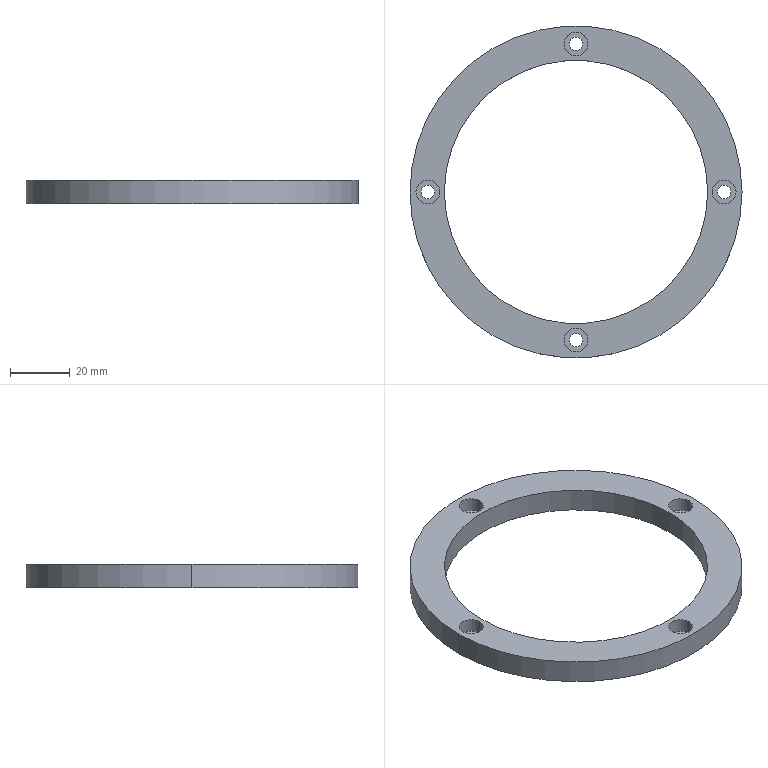Part | SolidWorks | features CirPattern 1, Extrusion 1, HoleWzd 1 | 1 solid | 26 faces | box 111 x 111 x 8 mm | volume 27617 mm3 | cylinder 20 | plane 6 | commonest cylinder face diameters 4.5 x8 8 x8 88 x2 111 x2
STEP:
#1=CARTESIAN_POINT('',(-53.5,0.,3.4));
#2=VERTEX_POINT('',#1);
#3=CARTESIAN_POINT('',(-45.5,0.,3.4));
#4=VERTEX_POINT('',#3);
#5=CARTESIAN_POINT('',(-49.5,0.,3.4));
#6=DIRECTION('',(0.,0.,1.));
#7=DIRECTION('',(1.,0.,0.));
#8=AXIS2_PLACEMENT_3D('',#5,#6,#7);
#9=CIRCLE('',#8,4.);
#10=EDGE_CURVE('',#2,#4,#9,.T.);
#11=ORIENTED_EDGE('',*,*,#10,.F.);
#12=CARTESIAN_POINT('',(-53.5,0.,8.));
#13=VERTEX_POINT('',#12);
#14=CARTESIAN_POINT('',(-53.5,0.,8.));
#15=DIRECTION('',(0.,0.,1.));
#16=VECTOR('',#15,1000.);
#17=LINE('',#14,#16);
#18=EDGE_CURVE('',#2,#13,#17,.T.);
#19=ORIENTED_EDGE('',*,*,#18,.T.);
#20=CARTESIAN_POINT('',(-45.5,0.,8.));
#21=VERTEX_POINT('',#20);
#22=CARTESIAN_POINT('',(-49.5,0.,8.));
#23=DIRECTION('',(0.,0.,1.));
#24=DIRECTION('',(1.,0.,0.));
#25=AXIS2_PLACEMENT_3D('',#22,#23,#24);
#26=CIRCLE('',#25,4.);
#27=EDGE_CURVE('',#13,#21,#26,.T.);
#28=ORIENTED_EDGE('',*,*,#27,.T.);
#29=CARTESIAN_POINT('',(-45.5,0.,8.));
#30=DIRECTION('',(0.,0.,1.));
#31=VECTOR('',#30,1000.);
#32=LINE('',#29,#31);
#33=EDGE_CURVE('',#4,#21,#32,.T.);
#34=ORIENTED_EDGE('',*,*,#33,.F.);
#35=EDGE_LOOP('',(#11,#19,#28,#34));
#36=FACE_OUTER_BOUND('',#35,.T.);
#37=CARTESIAN_POINT('',(-49.5,0.,8.));
#38=DIRECTION('',(0.,0.,1.));
#39=DIRECTION('',(1.,0.,0.));
#40=AXIS2_PLACEMENT_3D('',#37,#38,#39);
#41=CYLINDRICAL_SURFACE('',#40,4.);
#42=ADVANCED_FACE('',(#36),#41,.F.);
#43=CARTESIAN_POINT('',(-51.75,0.,0.));
#44=VERTEX_POINT('',#43);
#45=CARTESIAN_POINT('',(-47.25,0.,0.));
#46=VERTEX_POINT('',#45);
#47=CARTESIAN_POINT('',(-49.5,0.,0.));
#48=DIRECTION('',(0.,0.,1.));
#49=DIRECTION('',(1.,0.,0.));
#50=AXIS2_PLACEMENT_3D('',#47,#48,#49);
#51=CIRCLE('',#50,2.25);
#52=EDGE_CURVE('',#44,#46,#51,.T.);
#53=ORIENTED_EDGE('',*,*,#52,.F.);
#54=CARTESIAN_POINT('',(-51.75,0.,3.4));
#55=VERTEX_POINT('',#54);
#56=CARTESIAN_POINT('',(-51.75,0.,8.));
#57=DIRECTION('',(0.,0.,1.));
#58=VECTOR('',#57,1000.);
#59=LINE('',#56,#58);
#60=EDGE_CURVE('',#44,#55,#59,.T.);
#61=ORIENTED_EDGE('',*,*,#60,.T.);
#62=CARTESIAN_POINT('',(-47.25,0.,3.4));
#63=VERTEX_POINT('',#62);
#64=CARTESIAN_POINT('',(-49.5,0.,3.4));
#65=DIRECTION('',(0.,0.,1.));
#66=DIRECTION('',(1.,0.,0.));
#67=AXIS2_PLACEMENT_3D('',#64,#65,#66);
#68=CIRCLE('',#67,2.25);
#69=EDGE_CURVE('',#55,#63,#68,.T.);
#70=ORIENTED_EDGE('',*,*,#69,.T.);
#71=CARTESIAN_POINT('',(-47.25,0.,8.));
#72=DIRECTION('',(0.,0.,1.));
#73=VECTOR('',#72,1000.);
#74=LINE('',#71,#73);
#75=EDGE_CURVE('',#46,#63,#74,.T.);
#76=ORIENTED_EDGE('',*,*,#75,.F.);
#77=EDGE_LOOP('',(#53,#61,#70,#76));
#78=FACE_OUTER_BOUND('',#77,.T.);
#79=CARTESIAN_POINT('',(-49.5,0.,8.));
#80=DIRECTION('',(0.,0.,1.));
#81=DIRECTION('',(1.,0.,0.));
#82=AXIS2_PLACEMENT_3D('',#79,#80,#81);
#83=CYLINDRICAL_SURFACE('',#82,2.25);
#84=ADVANCED_FACE('',(#78),#83,.F.);
#85=CARTESIAN_POINT('',(-4.,-49.5,3.4));
#86=VERTEX_POINT('',#85);
#87=CARTESIAN_POINT('',(4.,-49.5,3.4));
#88=VERTEX_POINT('',#87);
#89=CARTESIAN_POINT('',(0.,-49.5,3.4));
#90=DIRECTION('',(0.,0.,1.));
#91=DIRECTION('',(1.,0.,0.));
#92=AXIS2_PLACEMENT_3D('',#89,#90,#91);
#93=CIRCLE('',#92,4.);
#94=EDGE_CURVE('',#86,#88,#93,.T.);
#95=ORIENTED_EDGE('',*,*,#94,.F.);
#96=CARTESIAN_POINT('',(-4.,-49.5,8.));
#97=VERTEX_POINT('',#96);
#98=CARTESIAN_POINT('',(-4.,-49.5,8.));
#99=DIRECTION('',(0.,0.,1.));
#100=VECTOR('',#99,1000.);
#101=LINE('',#98,#100);
#102=EDGE_CURVE('',#86,#97,#101,.T.);
#103=ORIENTED_EDGE('',*,*,#102,.T.);
#104=CARTESIAN_POINT('',(4.,-49.5,8.));
#105=VERTEX_POINT('',#104);
#106=CARTESIAN_POINT('',(0.,-49.5,8.));
#107=DIRECTION('',(0.,0.,1.));
#108=DIRECTION('',(1.,0.,0.));
#109=AXIS2_PLACEMENT_3D('',#106,#107,#108);
#110=CIRCLE('',#109,4.);
#111=EDGE_CURVE('',#97,#105,#110,.T.);
#112=ORIENTED_EDGE('',*,*,#111,.T.);
#113=CARTESIAN_POINT('',(4.,-49.5,8.));
#114=DIRECTION('',(0.,0.,1.));
#115=VECTOR('',#114,1000.);
#116=LINE('',#113,#115);
#117=EDGE_CURVE('',#88,#105,#116,.T.);
#118=ORIENTED_EDGE('',*,*,#117,.F.);
#119=EDGE_LOOP('',(#95,#103,#112,#118));
#120=FACE_OUTER_BOUND('',#119,.T.);
#121=CARTESIAN_POINT('',(0.,-49.5,8.));
#122=DIRECTION('',(0.,0.,1.));
#123=DIRECTION('',(1.,0.,0.));
#124=AXIS2_PLACEMENT_3D('',#121,#122,#123);
#125=CYLINDRICAL_SURFACE('',#124,4.);
#126=ADVANCED_FACE('',(#120),#125,.F.);
#127=CARTESIAN_POINT('',(-2.25,-49.5,0.));
#128=VERTEX_POINT('',#127);
#129=CARTESIAN_POINT('',(2.25,-49.5,0.));
#130=VERTEX_POINT('',#129);
#131=CARTESIAN_POINT('',(0.,-49.5,0.));
#132=DIRECTION('',(0.,0.,1.));
#133=DIRECTION('',(1.,0.,0.));
#134=AXIS2_PLACEMENT_3D('',#131,#132,#133);
#135=CIRCLE('',#134,2.25);
#136=EDGE_CURVE('',#128,#130,#135,.T.);
#137=ORIENTED_EDGE('',*,*,#136,.F.);
#138=CARTESIAN_POINT('',(-2.25,-49.5,3.4));
#139=VERTEX_POINT('',#138);
#140=CARTESIAN_POINT('',(-2.25,-49.5,8.));
#141=DIRECTION('',(0.,0.,1.));
#142=VECTOR('',#141,1000.);
#143=LINE('',#140,#142);
#144=EDGE_CURVE('',#128,#139,#143,.T.);
#145=ORIENTED_EDGE('',*,*,#144,.T.);
#146=CARTESIAN_POINT('',(2.25,-49.5,3.4));
#147=VERTEX_POINT('',#146);
#148=CARTESIAN_POINT('',(0.,-49.5,3.4));
#149=DIRECTION('',(0.,0.,1.));
#150=DIRECTION('',(1.,0.,0.));
#151=AXIS2_PLACEMENT_3D('',#148,#149,#150);
#152=CIRCLE('',#151,2.25);
#153=EDGE_CURVE('',#139,#147,#152,.T.);
#154=ORIENTED_EDGE('',*,*,#153,.T.);
#155=CARTESIAN_POINT('',(2.25,-49.5,8.));
#156=DIRECTION('',(0.,0.,1.));
#157=VECTOR('',#156,1000.);
#158=LINE('',#155,#157);
#159=EDGE_CURVE('',#130,#147,#158,.T.);
#160=ORIENTED_EDGE('',*,*,#159,.F.);
#161=EDGE_LOOP('',(#137,#145,#154,#160));
#162=FACE_OUTER_BOUND('',#161,.T.);
#163=CARTESIAN_POINT('',(0.,-49.5,8.));
#164=DIRECTION('',(0.,0.,1.));
#165=DIRECTION('',(1.,0.,0.));
#166=AXIS2_PLACEMENT_3D('',#163,#164,#165);
#167=CYLINDRICAL_SURFACE('',#166,2.25);
#168=ADVANCED_FACE('',(#162),#167,.F.);
#169=CARTESIAN_POINT('',(45.5,0.,3.4));
#170=VERTEX_POINT('',#169);
#171=CARTESIAN_POINT('',(53.5,0.,3.4));
#172=VERTEX_POINT('',#171);
#173=CARTESIAN_POINT('',(49.5,0.,3.4));
#174=DIRECTION('',(0.,0.,1.));
#175=DIRECTION('',(1.,0.,0.));
#176=AXIS2_PLACEMENT_3D('',#173,#174,#175);
#177=CIRCLE('',#176,4.);
#178=EDGE_CURVE('',#170,#172,#177,.T.);
#179=ORIENTED_EDGE('',*,*,#178,.F.);
#180=CARTESIAN_POINT('',(45.5,0.,8.));
#181=VERTEX_POINT('',#180);
#182=CARTESIAN_POINT('',(45.5,0.,8.));
#183=DIRECTION('',(0.,0.,1.));
#184=VECTOR('',#183,1000.);
#185=LINE('',#182,#184);
#186=EDGE_CURVE('',#170,#181,#185,.T.);
#187=ORIENTED_EDGE('',*,*,#186,.T.);
#188=CARTESIAN_POINT('',(53.5,0.,8.));
#189=VERTEX_POINT('',#188);
#190=CARTESIAN_POINT('',(49.5,0.,8.));
#191=DIRECTION('',(0.,0.,1.));
#192=DIRECTION('',(1.,0.,0.));
#193=AXIS2_PLACEMENT_3D('',#190,#191,#192);
#194=CIRCLE('',#193,4.);
#195=EDGE_CURVE('',#181,#189,#194,.T.);
#196=ORIENTED_EDGE('',*,*,#195,.T.);
#197=CARTESIAN_POINT('',(53.5,0.,8.));
#198=DIRECTION('',(0.,0.,1.));
#199=VECTOR('',#198,1000.);
#200=LINE('',#197,#199);
#201=EDGE_CURVE('',#172,#189,#200,.T.);
#202=ORIENTED_EDGE('',*,*,#201,.F.);
#203=EDGE_LOOP('',(#179,#187,#196,#202));
#204=FACE_OUTER_BOUND('',#203,.T.);
#205=CARTESIAN_POINT('',(49.5,0.,8.));
#206=DIRECTION('',(0.,0.,1.));
#207=DIRECTION('',(1.,0.,0.));
#208=AXIS2_PLACEMENT_3D('',#205,#206,#207);
#209=CYLINDRICAL_SURFACE('',#208,4.);
#210=ADVANCED_FACE('',(#204),#209,.F.);
#211=CARTESIAN_POINT('',(47.25,0.,0.));
#212=VERTEX_POINT('',#211);
#213=CARTESIAN_POINT('',(51.75,0.,0.));
#214=VERTEX_POINT('',#213);
#215=CARTESIAN_POINT('',(49.5,0.,0.));
#216=DIRECTION('',(0.,0.,1.));
#217=DIRECTION('',(1.,0.,0.));
#218=AXIS2_PLACEMENT_3D('',#215,#216,#217);
#219=CIRCLE('',#218,2.25);
#220=EDGE_CURVE('',#212,#214,#219,.T.);
#221=ORIENTED_EDGE('',*,*,#220,.F.);
#222=CARTESIAN_POINT('',(47.25,0.,3.4));
#223=VERTEX_POINT('',#222);
#224=CARTESIAN_POINT('',(47.25,0.,8.));
#225=DIRECTION('',(0.,0.,1.));
#226=VECTOR('',#225,1000.);
#227=LINE('',#224,#226);
#228=EDGE_CURVE('',#212,#223,#227,.T.);
#229=ORIENTED_EDGE('',*,*,#228,.T.);
#230=CARTESIAN_POINT('',(51.75,0.,3.4));
#231=VERTEX_POINT('',#230);
#232=CARTESIAN_POINT('',(49.5,0.,3.4));
#233=DIRECTION('',(0.,0.,1.));
#234=DIRECTION('',(1.,0.,0.));
#235=AXIS2_PLACEMENT_3D('',#232,#233,#234);
#236=CIRCLE('',#235,2.25);
#237=EDGE_CURVE('',#223,#231,#236,.T.);
#238=ORIENTED_EDGE('',*,*,#237,.T.);
#239=CARTESIAN_POINT('',(51.75,0.,8.));
#240=DIRECTION('',(0.,0.,1.));
#241=VECTOR('',#240,1000.);
#242=LINE('',#239,#241);
#243=EDGE_CURVE('',#214,#231,#242,.T.);
#244=ORIENTED_EDGE('',*,*,#243,.F.);
#245=EDGE_LOOP('',(#221,#229,#238,#244));
#246=FACE_OUTER_BOUND('',#245,.T.);
#247=CARTESIAN_POINT('',(49.5,0.,8.));
#248=DIRECTION('',(0.,0.,1.));
#249=DIRECTION('',(1.,0.,0.));
#250=AXIS2_PLACEMENT_3D('',#247,#248,#249);
#251=CYLINDRICAL_SURFACE('',#250,2.25);
#252=ADVANCED_FACE('',(#246),#251,.F.);
#253=CARTESIAN_POINT('',(-4.,49.5,3.4));
#254=VERTEX_POINT('',#253);
#255=CARTESIAN_POINT('',(4.,49.5,3.4));
#256=VERTEX_POINT('',#255);
#257=CARTESIAN_POINT('',(0.,49.5,3.4));
#258=DIRECTION('',(0.,0.,1.));
#259=DIRECTION('',(1.,0.,0.));
#260=AXIS2_PLACEMENT_3D('',#257,#258,#259);
#261=CIRCLE('',#260,4.);
#262=EDGE_CURVE('',#254,#256,#261,.T.);
#263=ORIENTED_EDGE('',*,*,#262,.F.);
#264=CARTESIAN_POINT('',(-4.,49.5,8.));
#265=VERTEX_POINT('',#264);
#266=CARTESIAN_POINT('',(-4.,49.5,8.));
#267=DIRECTION('',(0.,0.,1.));
#268=VECTOR('',#267,1000.);
#269=LINE('',#266,#268);
#270=EDGE_CURVE('',#254,#265,#269,.T.);
#271=ORIENTED_EDGE('',*,*,#270,.T.);
#272=CARTESIAN_POINT('',(4.,49.5,8.));
#273=VERTEX_POINT('',#272);
#274=CARTESIAN_POINT('',(0.,49.5,8.));
#275=DIRECTION('',(0.,0.,1.));
#276=DIRECTION('',(1.,0.,0.));
#277=AXIS2_PLACEMENT_3D('',#274,#275,#276);
#278=CIRCLE('',#277,4.);
#279=EDGE_CURVE('',#265,#273,#278,.T.);
#280=ORIENTED_EDGE('',*,*,#279,.T.);
#281=CARTESIAN_POINT('',(4.,49.5,8.));
#282=DIRECTION('',(0.,0.,1.));
#283=VECTOR('',#282,1000.);
#284=LINE('',#281,#283);
#285=EDGE_CURVE('',#256,#273,#284,.T.);
#286=ORIENTED_EDGE('',*,*,#285,.F.);
#287=EDGE_LOOP('',(#263,#271,#280,#286));
#288=FACE_OUTER_BOUND('',#287,.T.);
#289=CARTESIAN_POINT('',(0.,49.5,8.));
#290=DIRECTION('',(0.,0.,1.));
#291=DIRECTION('',(1.,0.,0.));
#292=AXIS2_PLACEMENT_3D('',#289,#290,#291);
#293=CYLINDRICAL_SURFACE('',#292,4.);
#294=ADVANCED_FACE('',(#288),#293,.F.);
#295=CARTESIAN_POINT('',(-2.25,49.5,0.));
#296=VERTEX_POINT('',#295);
#297=CARTESIAN_POINT('',(2.25,49.5,0.));
#298=VERTEX_POINT('',#297);
#299=CARTESIAN_POINT('',(0.,49.5,0.));
#300=DIRECTION('',(0.,0.,1.));
#301=DIRECTION('',(1.,0.,0.));
#302=AXIS2_PLACEMENT_3D('',#299,#300,#301);
#303=CIRCLE('',#302,2.25);
#304=EDGE_CURVE('',#296,#298,#303,.T.);
#305=ORIENTED_EDGE('',*,*,#304,.F.);
#306=CARTESIAN_POINT('',(-2.25,49.5,3.4));
#307=VERTEX_POINT('',#306);
#308=CARTESIAN_POINT('',(-2.25,49.5,8.));
#309=DIRECTION('',(0.,0.,1.));
#310=VECTOR('',#309,1000.);
#311=LINE('',#308,#310);
#312=EDGE_CURVE('',#296,#307,#311,.T.);
#313=ORIENTED_EDGE('',*,*,#312,.T.);
#314=CARTESIAN_POINT('',(2.25,49.5,3.4));
#315=VERTEX_POINT('',#314);
#316=CARTESIAN_POINT('',(0.,49.5,3.4));
#317=DIRECTION('',(0.,0.,1.));
#318=DIRECTION('',(1.,0.,0.));
#319=AXIS2_PLACEMENT_3D('',#316,#317,#318);
#320=CIRCLE('',#319,2.25);
#321=EDGE_CURVE('',#307,#315,#320,.T.);
#322=ORIENTED_EDGE('',*,*,#321,.T.);
#323=CARTESIAN_POINT('',(2.25,49.5,8.));
#324=DIRECTION('',(0.,0.,1.));
#325=VECTOR('',#324,1000.);
#326=LINE('',#323,#325);
#327=EDGE_CURVE('',#298,#315,#326,.T.);
#328=ORIENTED_EDGE('',*,*,#327,.F.);
#329=EDGE_LOOP('',(#305,#313,#322,#328));
#330=FACE_OUTER_BOUND('',#329,.T.);
#331=CARTESIAN_POINT('',(0.,49.5,8.));
#332=DIRECTION('',(0.,0.,1.));
#333=DIRECTION('',(1.,0.,0.));
#334=AXIS2_PLACEMENT_3D('',#331,#332,#333);
#335=CYLINDRICAL_SURFACE('',#334,2.25);
#336=ADVANCED_FACE('',(#330),#335,.F.);
#337=CARTESIAN_POINT('',(-44.,0.,8.));
#338=VERTEX_POINT('',#337);
#339=CARTESIAN_POINT('',(44.,0.,8.));
#340=VERTEX_POINT('',#339);
#341=CARTESIAN_POINT('',(0.,0.,8.));
#342=DIRECTION('',(0.,0.,1.));
#343=DIRECTION('',(1.,0.,0.));
#344=AXIS2_PLACEMENT_3D('',#341,#342,#343);
#345=CIRCLE('',#344,44.);
#346=EDGE_CURVE('',#338,#340,#345,.T.);
#347=ORIENTED_EDGE('',*,*,#346,.T.);
#348=CARTESIAN_POINT('',(44.,0.,0.));
#349=VERTEX_POINT('',#348);
#350=CARTESIAN_POINT('',(44.,0.,8.));
#351=DIRECTION('',(0.,0.,-1.));
#352=VECTOR('',#351,1000.);
#353=LINE('',#350,#352);
#354=EDGE_CURVE('',#340,#349,#353,.T.);
#355=ORIENTED_EDGE('',*,*,#354,.T.);
#356=CARTESIAN_POINT('',(-44.,0.,0.));
#357=VERTEX_POINT('',#356);
#358=CARTESIAN_POINT('',(0.,0.,0.));
#359=DIRECTION('',(0.,0.,1.));
#360=DIRECTION('',(1.,0.,0.));
#361=AXIS2_PLACEMENT_3D('',#358,#359,#360);
#362=CIRCLE('',#361,44.);
#363=EDGE_CURVE('',#357,#349,#362,.T.);
#364=ORIENTED_EDGE('',*,*,#363,.F.);
#365=CARTESIAN_POINT('',(-44.,0.,8.));
#366=DIRECTION('',(0.,0.,-1.));
#367=VECTOR('',#366,1000.);
#368=LINE('',#365,#367);
#369=EDGE_CURVE('',#338,#357,#368,.T.);
#370=ORIENTED_EDGE('',*,*,#369,.F.);
#371=EDGE_LOOP('',(#347,#355,#364,#370));
#372=FACE_OUTER_BOUND('',#371,.T.);
#373=CARTESIAN_POINT('',(0.,0.,8.));
#374=DIRECTION('',(0.,0.,-1.));
#375=DIRECTION('',(-1.,0.,0.));
#376=AXIS2_PLACEMENT_3D('',#373,#374,#375);
#377=CYLINDRICAL_SURFACE('',#376,44.);
#378=ADVANCED_FACE('',(#372),#377,.F.);
#379=CARTESIAN_POINT('',(55.5,0.,8.));
#380=VERTEX_POINT('',#379);
#381=CARTESIAN_POINT('',(-55.5,0.,8.));
#382=VERTEX_POINT('',#381);
#383=CARTESIAN_POINT('',(0.,0.,8.));
#384=DIRECTION('',(0.,0.,1.));
#385=DIRECTION('',(1.,0.,0.));
#386=AXIS2_PLACEMENT_3D('',#383,#384,#385);
#387=CIRCLE('',#386,55.5);
#388=EDGE_CURVE('',#380,#382,#387,.T.);
#389=ORIENTED_EDGE('',*,*,#388,.F.);
#390=CARTESIAN_POINT('',(55.5,0.,0.));
#391=VERTEX_POINT('',#390);
#392=CARTESIAN_POINT('',(55.5,0.,8.));
#393=DIRECTION('',(0.,0.,-1.));
#394=VECTOR('',#393,1000.);
#395=LINE('',#392,#394);
#396=EDGE_CURVE('',#380,#391,#395,.T.);
#397=ORIENTED_EDGE('',*,*,#396,.T.);
#398=CARTESIAN_POINT('',(-55.5,0.,0.));
#399=VERTEX_POINT('',#398);
#400=CARTESIAN_POINT('',(0.,0.,0.));
#401=DIRECTION('',(0.,0.,1.));
#402=DIRECTION('',(1.,0.,0.));
#403=AXIS2_PLACEMENT_3D('',#400,#401,#402);
#404=CIRCLE('',#403,55.5);
#405=EDGE_CURVE('',#391,#399,#404,.T.);
#406=ORIENTED_EDGE('',*,*,#405,.T.);
#407=CARTESIAN_POINT('',(-55.5,0.,8.));
#408=DIRECTION('',(0.,0.,-1.));
#409=VECTOR('',#408,1000.);
#410=LINE('',#407,#409);
#411=EDGE_CURVE('',#382,#399,#410,.T.);
#412=ORIENTED_EDGE('',*,*,#411,.F.);
#413=EDGE_LOOP('',(#389,#397,#406,#412));
#414=FACE_OUTER_BOUND('',#413,.T.);
#415=CARTESIAN_POINT('',(0.,0.,8.));
#416=DIRECTION('',(0.,0.,-1.));
#417=DIRECTION('',(-1.,0.,0.));
#418=AXIS2_PLACEMENT_3D('',#415,#416,#417);
#419=CYLINDRICAL_SURFACE('',#418,55.5);
#420=ADVANCED_FACE('',(#414),#419,.T.);
#421=CARTESIAN_POINT('',(-49.5,0.,8.));
#422=DIRECTION('',(0.,0.,1.));
#423=DIRECTION('',(1.,0.,0.));
#424=AXIS2_PLACEMENT_3D('',#421,#422,#423);
#425=CIRCLE('',#424,4.);
#426=EDGE_CURVE('',#21,#13,#425,.T.);
#427=ORIENTED_EDGE('',*,*,#426,.F.);
#428=ORIENTED_EDGE('',*,*,#27,.F.);
#429=EDGE_LOOP('',(#427,#428));
#430=FACE_BOUND('',#429,.T.);
#431=CARTESIAN_POINT('',(0.,-49.5,8.));
#432=DIRECTION('',(0.,0.,1.));
#433=DIRECTION('',(1.,0.,0.));
#434=AXIS2_PLACEMENT_3D('',#431,#432,#433);
#435=CIRCLE('',#434,4.);
#436=EDGE_CURVE('',#105,#97,#435,.T.);
#437=ORIENTED_EDGE('',*,*,#436,.F.);
#438=ORIENTED_EDGE('',*,*,#111,.F.);
#439=EDGE_LOOP('',(#437,#438));
#440=FACE_BOUND('',#439,.T.);
#441=CARTESIAN_POINT('',(49.5,0.,8.));
#442=DIRECTION('',(0.,0.,1.));
#443=DIRECTION('',(1.,0.,0.));
#444=AXIS2_PLACEMENT_3D('',#441,#442,#443);
#445=CIRCLE('',#444,4.);
#446=EDGE_CURVE('',#189,#181,#445,.T.);
#447=ORIENTED_EDGE('',*,*,#446,.F.);
#448=ORIENTED_EDGE('',*,*,#195,.F.);
#449=EDGE_LOOP('',(#447,#448));
#450=FACE_BOUND('',#449,.T.);
#451=CARTESIAN_POINT('',(0.,49.5,8.));
#452=DIRECTION('',(0.,0.,1.));
#453=DIRECTION('',(1.,0.,0.));
#454=AXIS2_PLACEMENT_3D('',#451,#452,#453);
#455=CIRCLE('',#454,4.);
#456=EDGE_CURVE('',#273,#265,#455,.T.);
#457=ORIENTED_EDGE('',*,*,#456,.F.);
#458=ORIENTED_EDGE('',*,*,#279,.F.);
#459=EDGE_LOOP('',(#457,#458));
#460=FACE_BOUND('',#459,.T.);
#461=CARTESIAN_POINT('',(0.,0.,8.));
#462=DIRECTION('',(0.,0.,1.));
#463=DIRECTION('',(1.,0.,0.));
#464=AXIS2_PLACEMENT_3D('',#461,#462,#463);
#465=CIRCLE('',#464,55.5);
#466=EDGE_CURVE('',#382,#380,#465,.T.);
#467=ORIENTED_EDGE('',*,*,#466,.T.);
#468=ORIENTED_EDGE('',*,*,#388,.T.);
#469=EDGE_LOOP('',(#467,#468));
#470=FACE_OUTER_BOUND('',#469,.T.);
#471=ORIENTED_EDGE('',*,*,#346,.F.);
#472=CARTESIAN_POINT('',(0.,0.,8.));
#473=DIRECTION('',(0.,0.,1.));
#474=DIRECTION('',(1.,0.,0.));
#475=AXIS2_PLACEMENT_3D('',#472,#473,#474);
#476=CIRCLE('',#475,44.);
#477=EDGE_CURVE('',#340,#338,#476,.T.);
#478=ORIENTED_EDGE('',*,*,#477,.F.);
#479=EDGE_LOOP('',(#471,#478));
#480=FACE_BOUND('',#479,.T.);
#481=CARTESIAN_POINT('',(0.,0.,8.));
#482=DIRECTION('',(0.,0.,1.));
#483=DIRECTION('',(1.,0.,0.));
#484=AXIS2_PLACEMENT_3D('',#481,#482,#483);
#485=PLANE('',#484);
#486=ADVANCED_FACE('',(#430,#440,#450,#460,#470,#480),#485,.T.);
#487=CARTESIAN_POINT('',(-49.5,0.,0.));
#488=DIRECTION('',(0.,0.,1.));
#489=DIRECTION('',(1.,0.,0.));
#490=AXIS2_PLACEMENT_3D('',#487,#488,#489);
#491=CIRCLE('',#490,2.25);
#492=EDGE_CURVE('',#46,#44,#491,.T.);
#493=ORIENTED_EDGE('',*,*,#492,.T.);
#494=ORIENTED_EDGE('',*,*,#52,.T.);
#495=EDGE_LOOP('',(#493,#494));
#496=FACE_BOUND('',#495,.T.);
#497=CARTESIAN_POINT('',(0.,-49.5,0.));
#498=DIRECTION('',(0.,0.,1.));
#499=DIRECTION('',(1.,0.,0.));
#500=AXIS2_PLACEMENT_3D('',#497,#498,#499);
#501=CIRCLE('',#500,2.25);
#502=EDGE_CURVE('',#130,#128,#501,.T.);
#503=ORIENTED_EDGE('',*,*,#502,.T.);
#504=ORIENTED_EDGE('',*,*,#136,.T.);
#505=EDGE_LOOP('',(#503,#504));
#506=FACE_BOUND('',#505,.T.);
#507=CARTESIAN_POINT('',(49.5,0.,0.));
#508=DIRECTION('',(0.,0.,1.));
#509=DIRECTION('',(1.,0.,0.));
#510=AXIS2_PLACEMENT_3D('',#507,#508,#509);
#511=CIRCLE('',#510,2.25);
#512=EDGE_CURVE('',#214,#212,#511,.T.);
#513=ORIENTED_EDGE('',*,*,#512,.T.);
#514=ORIENTED_EDGE('',*,*,#220,.T.);
#515=EDGE_LOOP('',(#513,#514));
#516=FACE_BOUND('',#515,.T.);
#517=CARTESIAN_POINT('',(0.,49.5,0.));
#518=DIRECTION('',(0.,0.,1.));
#519=DIRECTION('',(1.,0.,0.));
#520=AXIS2_PLACEMENT_3D('',#517,#518,#519);
#521=CIRCLE('',#520,2.25);
#522=EDGE_CURVE('',#298,#296,#521,.T.);
#523=ORIENTED_EDGE('',*,*,#522,.T.);
#524=ORIENTED_EDGE('',*,*,#304,.T.);
#525=EDGE_LOOP('',(#523,#524));
#526=FACE_BOUND('',#525,.T.);
#527=CARTESIAN_POINT('',(0.,0.,0.));
#528=DIRECTION('',(0.,0.,1.));
#529=DIRECTION('',(1.,0.,0.));
#530=AXIS2_PLACEMENT_3D('',#527,#528,#529);
#531=CIRCLE('',#530,55.5);
#532=EDGE_CURVE('',#399,#391,#531,.T.);
#533=ORIENTED_EDGE('',*,*,#532,.F.);
#534=ORIENTED_EDGE('',*,*,#405,.F.);
#535=EDGE_LOOP('',(#533,#534));
#536=FACE_OUTER_BOUND('',#535,.T.);
#537=ORIENTED_EDGE('',*,*,#363,.T.);
#538=CARTESIAN_POINT('',(0.,0.,0.));
#539=DIRECTION('',(0.,0.,1.));
#540=DIRECTION('',(1.,0.,0.));
#541=AXIS2_PLACEMENT_3D('',#538,#539,#540);
#542=CIRCLE('',#541,44.);
#543=EDGE_CURVE('',#349,#357,#542,.T.);
#544=ORIENTED_EDGE('',*,*,#543,.T.);
#545=EDGE_LOOP('',(#537,#544));
#546=FACE_BOUND('',#545,.T.);
#547=CARTESIAN_POINT('',(0.,0.,0.));
#548=DIRECTION('',(0.,0.,1.));
#549=DIRECTION('',(1.,0.,0.));
#550=AXIS2_PLACEMENT_3D('',#547,#548,#549);
#551=PLANE('',#550);
#552=ADVANCED_FACE('',(#496,#506,#516,#526,#536,#546),#551,.F.);
#553=ORIENTED_EDGE('',*,*,#396,.F.);
#554=ORIENTED_EDGE('',*,*,#466,.F.);
#555=ORIENTED_EDGE('',*,*,#411,.T.);
#556=ORIENTED_EDGE('',*,*,#532,.T.);
#557=EDGE_LOOP('',(#553,#554,#555,#556));
#558=FACE_OUTER_BOUND('',#557,.T.);
#559=CARTESIAN_POINT('',(0.,0.,8.));
#560=DIRECTION('',(0.,0.,-1.));
#561=DIRECTION('',(-1.,0.,0.));
#562=AXIS2_PLACEMENT_3D('',#559,#560,#561);
#563=CYLINDRICAL_SURFACE('',#562,55.5);
#564=ADVANCED_FACE('',(#558),#563,.T.);
#565=ORIENTED_EDGE('',*,*,#354,.F.);
#566=ORIENTED_EDGE('',*,*,#477,.T.);
#567=ORIENTED_EDGE('',*,*,#369,.T.);
#568=ORIENTED_EDGE('',*,*,#543,.F.);
#569=EDGE_LOOP('',(#565,#566,#567,#568));
#570=FACE_OUTER_BOUND('',#569,.T.);
#571=CARTESIAN_POINT('',(0.,0.,8.));
#572=DIRECTION('',(0.,0.,-1.));
#573=DIRECTION('',(-1.,0.,0.));
#574=AXIS2_PLACEMENT_3D('',#571,#572,#573);
#575=CYLINDRICAL_SURFACE('',#574,44.);
#576=ADVANCED_FACE('',(#570),#575,.F.);
#577=ORIENTED_EDGE('',*,*,#312,.F.);
#578=ORIENTED_EDGE('',*,*,#522,.F.);
#579=ORIENTED_EDGE('',*,*,#327,.T.);
#580=CARTESIAN_POINT('',(0.,49.5,3.4));
#581=DIRECTION('',(0.,0.,1.));
#582=DIRECTION('',(1.,0.,0.));
#583=AXIS2_PLACEMENT_3D('',#580,#581,#582);
#584=CIRCLE('',#583,2.25);
#585=EDGE_CURVE('',#315,#307,#584,.T.);
#586=ORIENTED_EDGE('',*,*,#585,.T.);
#587=EDGE_LOOP('',(#577,#578,#579,#586));
#588=FACE_OUTER_BOUND('',#587,.T.);
#589=CARTESIAN_POINT('',(0.,49.5,8.));
#590=DIRECTION('',(0.,0.,1.));
#591=DIRECTION('',(1.,0.,0.));
#592=AXIS2_PLACEMENT_3D('',#589,#590,#591);
#593=CYLINDRICAL_SURFACE('',#592,2.25);
#594=ADVANCED_FACE('',(#588),#593,.F.);
#595=ORIENTED_EDGE('',*,*,#585,.F.);
#596=ORIENTED_EDGE('',*,*,#321,.F.);
#597=EDGE_LOOP('',(#595,#596));
#598=FACE_BOUND('',#597,.T.);
#599=CARTESIAN_POINT('',(0.,49.5,3.4));
#600=DIRECTION('',(0.,0.,1.));
#601=DIRECTION('',(1.,0.,0.));
#602=AXIS2_PLACEMENT_3D('',#599,#600,#601);
#603=CIRCLE('',#602,4.);
#604=EDGE_CURVE('',#256,#254,#603,.T.);
#605=ORIENTED_EDGE('',*,*,#604,.T.);
#606=ORIENTED_EDGE('',*,*,#262,.T.);
#607=EDGE_LOOP('',(#605,#606));
#608=FACE_OUTER_BOUND('',#607,.T.);
#609=CARTESIAN_POINT('',(2.25,49.5,3.4));
#610=DIRECTION('',(0.,0.,-1.));
#611=DIRECTION('',(-1.,0.,0.));
#612=AXIS2_PLACEMENT_3D('',#609,#610,#611);
#613=PLANE('',#612);
#614=ADVANCED_FACE('',(#598,#608),#613,.F.);
#615=ORIENTED_EDGE('',*,*,#270,.F.);
#616=ORIENTED_EDGE('',*,*,#604,.F.);
#617=ORIENTED_EDGE('',*,*,#285,.T.);
#618=ORIENTED_EDGE('',*,*,#456,.T.);
#619=EDGE_LOOP('',(#615,#616,#617,#618));
#620=FACE_OUTER_BOUND('',#619,.T.);
#621=CARTESIAN_POINT('',(0.,49.5,8.));
#622=DIRECTION('',(0.,0.,1.));
#623=DIRECTION('',(1.,0.,0.));
#624=AXIS2_PLACEMENT_3D('',#621,#622,#623);
#625=CYLINDRICAL_SURFACE('',#624,4.);
#626=ADVANCED_FACE('',(#620),#625,.F.);
#627=ORIENTED_EDGE('',*,*,#228,.F.);
#628=ORIENTED_EDGE('',*,*,#512,.F.);
#629=ORIENTED_EDGE('',*,*,#243,.T.);
#630=CARTESIAN_POINT('',(49.5,0.,3.4));
#631=DIRECTION('',(0.,0.,1.));
#632=DIRECTION('',(1.,0.,0.));
#633=AXIS2_PLACEMENT_3D('',#630,#631,#632);
#634=CIRCLE('',#633,2.25);
#635=EDGE_CURVE('',#231,#223,#634,.T.);
#636=ORIENTED_EDGE('',*,*,#635,.T.);
#637=EDGE_LOOP('',(#627,#628,#629,#636));
#638=FACE_OUTER_BOUND('',#637,.T.);
#639=CARTESIAN_POINT('',(49.5,0.,8.));
#640=DIRECTION('',(0.,0.,1.));
#641=DIRECTION('',(1.,0.,0.));
#642=AXIS2_PLACEMENT_3D('',#639,#640,#641);
#643=CYLINDRICAL_SURFACE('',#642,2.25);
#644=ADVANCED_FACE('',(#638),#643,.F.);
#645=ORIENTED_EDGE('',*,*,#635,.F.);
#646=ORIENTED_EDGE('',*,*,#237,.F.);
#647=EDGE_LOOP('',(#645,#646));
#648=FACE_BOUND('',#647,.T.);
#649=CARTESIAN_POINT('',(49.5,0.,3.4));
#650=DIRECTION('',(0.,0.,1.));
#651=DIRECTION('',(1.,0.,0.));
#652=AXIS2_PLACEMENT_3D('',#649,#650,#651);
#653=CIRCLE('',#652,4.);
#654=EDGE_CURVE('',#172,#170,#653,.T.);
#655=ORIENTED_EDGE('',*,*,#654,.T.);
#656=ORIENTED_EDGE('',*,*,#178,.T.);
#657=EDGE_LOOP('',(#655,#656));
#658=FACE_OUTER_BOUND('',#657,.T.);
#659=CARTESIAN_POINT('',(51.75,0.,3.4));
#660=DIRECTION('',(0.,0.,-1.));
#661=DIRECTION('',(-1.,0.,0.));
#662=AXIS2_PLACEMENT_3D('',#659,#660,#661);
#663=PLANE('',#662);
#664=ADVANCED_FACE('',(#648,#658),#663,.F.);
#665=ORIENTED_EDGE('',*,*,#186,.F.);
#666=ORIENTED_EDGE('',*,*,#654,.F.);
#667=ORIENTED_EDGE('',*,*,#201,.T.);
#668=ORIENTED_EDGE('',*,*,#446,.T.);
#669=EDGE_LOOP('',(#665,#666,#667,#668));
#670=FACE_OUTER_BOUND('',#669,.T.);
#671=CARTESIAN_POINT('',(49.5,0.,8.));
#672=DIRECTION('',(0.,0.,1.));
#673=DIRECTION('',(1.,0.,0.));
#674=AXIS2_PLACEMENT_3D('',#671,#672,#673);
#675=CYLINDRICAL_SURFACE('',#674,4.);
#676=ADVANCED_FACE('',(#670),#675,.F.);
#677=ORIENTED_EDGE('',*,*,#144,.F.);
#678=ORIENTED_EDGE('',*,*,#502,.F.);
#679=ORIENTED_EDGE('',*,*,#159,.T.);
#680=CARTESIAN_POINT('',(0.,-49.5,3.4));
#681=DIRECTION('',(0.,0.,1.));
#682=DIRECTION('',(1.,0.,0.));
#683=AXIS2_PLACEMENT_3D('',#680,#681,#682);
#684=CIRCLE('',#683,2.25);
#685=EDGE_CURVE('',#147,#139,#684,.T.);
#686=ORIENTED_EDGE('',*,*,#685,.T.);
#687=EDGE_LOOP('',(#677,#678,#679,#686));
#688=FACE_OUTER_BOUND('',#687,.T.);
#689=CARTESIAN_POINT('',(0.,-49.5,8.));
#690=DIRECTION('',(0.,0.,1.));
#691=DIRECTION('',(1.,0.,0.));
#692=AXIS2_PLACEMENT_3D('',#689,#690,#691);
#693=CYLINDRICAL_SURFACE('',#692,2.25);
#694=ADVANCED_FACE('',(#688),#693,.F.);
#695=ORIENTED_EDGE('',*,*,#685,.F.);
#696=ORIENTED_EDGE('',*,*,#153,.F.);
#697=EDGE_LOOP('',(#695,#696));
#698=FACE_BOUND('',#697,.T.);
#699=CARTESIAN_POINT('',(0.,-49.5,3.4));
#700=DIRECTION('',(0.,0.,1.));
#701=DIRECTION('',(1.,0.,0.));
#702=AXIS2_PLACEMENT_3D('',#699,#700,#701);
#703=CIRCLE('',#702,4.);
#704=EDGE_CURVE('',#88,#86,#703,.T.);
#705=ORIENTED_EDGE('',*,*,#704,.T.);
#706=ORIENTED_EDGE('',*,*,#94,.T.);
#707=EDGE_LOOP('',(#705,#706));
#708=FACE_OUTER_BOUND('',#707,.T.);
#709=CARTESIAN_POINT('',(2.25,-49.5,3.4));
#710=DIRECTION('',(0.,0.,-1.));
#711=DIRECTION('',(-1.,0.,0.));
#712=AXIS2_PLACEMENT_3D('',#709,#710,#711);
#713=PLANE('',#712);
#714=ADVANCED_FACE('',(#698,#708),#713,.F.);
#715=ORIENTED_EDGE('',*,*,#102,.F.);
#716=ORIENTED_EDGE('',*,*,#704,.F.);
#717=ORIENTED_EDGE('',*,*,#117,.T.);
#718=ORIENTED_EDGE('',*,*,#436,.T.);
#719=EDGE_LOOP('',(#715,#716,#717,#718));
#720=FACE_OUTER_BOUND('',#719,.T.);
#721=CARTESIAN_POINT('',(0.,-49.5,8.));
#722=DIRECTION('',(0.,0.,1.));
#723=DIRECTION('',(1.,0.,0.));
#724=AXIS2_PLACEMENT_3D('',#721,#722,#723);
#725=CYLINDRICAL_SURFACE('',#724,4.);
#726=ADVANCED_FACE('',(#720),#725,.F.);
#727=ORIENTED_EDGE('',*,*,#60,.F.);
#728=ORIENTED_EDGE('',*,*,#492,.F.);
#729=ORIENTED_EDGE('',*,*,#75,.T.);
#730=CARTESIAN_POINT('',(-49.5,0.,3.4));
#731=DIRECTION('',(0.,0.,1.));
#732=DIRECTION('',(1.,0.,0.));
#733=AXIS2_PLACEMENT_3D('',#730,#731,#732);
#734=CIRCLE('',#733,2.25);
#735=EDGE_CURVE('',#63,#55,#734,.T.);
#736=ORIENTED_EDGE('',*,*,#735,.T.);
#737=EDGE_LOOP('',(#727,#728,#729,#736));
#738=FACE_OUTER_BOUND('',#737,.T.);
#739=CARTESIAN_POINT('',(-49.5,0.,8.));
#740=DIRECTION('',(0.,0.,1.));
#741=DIRECTION('',(1.,0.,0.));
#742=AXIS2_PLACEMENT_3D('',#739,#740,#741);
#743=CYLINDRICAL_SURFACE('',#742,2.25);
#744=ADVANCED_FACE('',(#738),#743,.F.);
#745=ORIENTED_EDGE('',*,*,#735,.F.);
#746=ORIENTED_EDGE('',*,*,#69,.F.);
#747=EDGE_LOOP('',(#745,#746));
#748=FACE_BOUND('',#747,.T.);
#749=CARTESIAN_POINT('',(-49.5,0.,3.4));
#750=DIRECTION('',(0.,0.,1.));
#751=DIRECTION('',(1.,0.,0.));
#752=AXIS2_PLACEMENT_3D('',#749,#750,#751);
#753=CIRCLE('',#752,4.);
#754=EDGE_CURVE('',#4,#2,#753,.T.);
#755=ORIENTED_EDGE('',*,*,#754,.T.);
#756=ORIENTED_EDGE('',*,*,#10,.T.);
#757=EDGE_LOOP('',(#755,#756));
#758=FACE_OUTER_BOUND('',#757,.T.);
#759=CARTESIAN_POINT('',(-47.25,0.,3.4));
#760=DIRECTION('',(0.,0.,-1.));
#761=DIRECTION('',(-1.,0.,0.));
#762=AXIS2_PLACEMENT_3D('',#759,#760,#761);
#763=PLANE('',#762);
#764=ADVANCED_FACE('',(#748,#758),#763,.F.);
#765=ORIENTED_EDGE('',*,*,#18,.F.);
#766=ORIENTED_EDGE('',*,*,#754,.F.);
#767=ORIENTED_EDGE('',*,*,#33,.T.);
#768=ORIENTED_EDGE('',*,*,#426,.T.);
#769=EDGE_LOOP('',(#765,#766,#767,#768));
#770=FACE_OUTER_BOUND('',#769,.T.);
#771=CARTESIAN_POINT('',(-49.5,0.,8.));
#772=DIRECTION('',(0.,0.,1.));
#773=DIRECTION('',(1.,0.,0.));
#774=AXIS2_PLACEMENT_3D('',#771,#772,#773);
#775=CYLINDRICAL_SURFACE('',#774,4.);
#776=ADVANCED_FACE('',(#770),#775,.F.);
#777=CLOSED_SHELL('',(#42,#84,#126,#168,#210,#252,#294,#336,#378,#420,#486,#552,#564,#576,#594,#614,#626,#644,#664,#676,#694,#714,#726,#744,#764,#776));
#778=MANIFOLD_SOLID_BREP('',#777);
#779=CARTESIAN_POINT('',(0.,0.,0.));
#780=DIRECTION('',(0.,0.,1.));
#781=DIRECTION('',(1.,0.,0.));
#782=AXIS2_PLACEMENT_3D('',#779,#780,#781);
#783=(LENGTH_UNIT()NAMED_UNIT(*)SI_UNIT(.MILLI.,.METRE.));
#784=UNCERTAINTY_MEASURE_WITH_UNIT(LENGTH_MEASURE(0.00001),#783,'','');
#785=(NAMED_UNIT(*)PLANE_ANGLE_UNIT()SI_UNIT($,.RADIAN.));
#786=(NAMED_UNIT(*)SI_UNIT($,.STERADIAN.)SOLID_ANGLE_UNIT());
#787=(GEOMETRIC_REPRESENTATION_CONTEXT(3)GLOBAL_UNCERTAINTY_ASSIGNED_CONTEXT((#784))GLOBAL_UNIT_ASSIGNED_CONTEXT((#783,#785,#786))REPRESENTATION_CONTEXT('',''));
#788=ADVANCED_BREP_SHAPE_REPRESENTATION('',(#778,#782),#787);